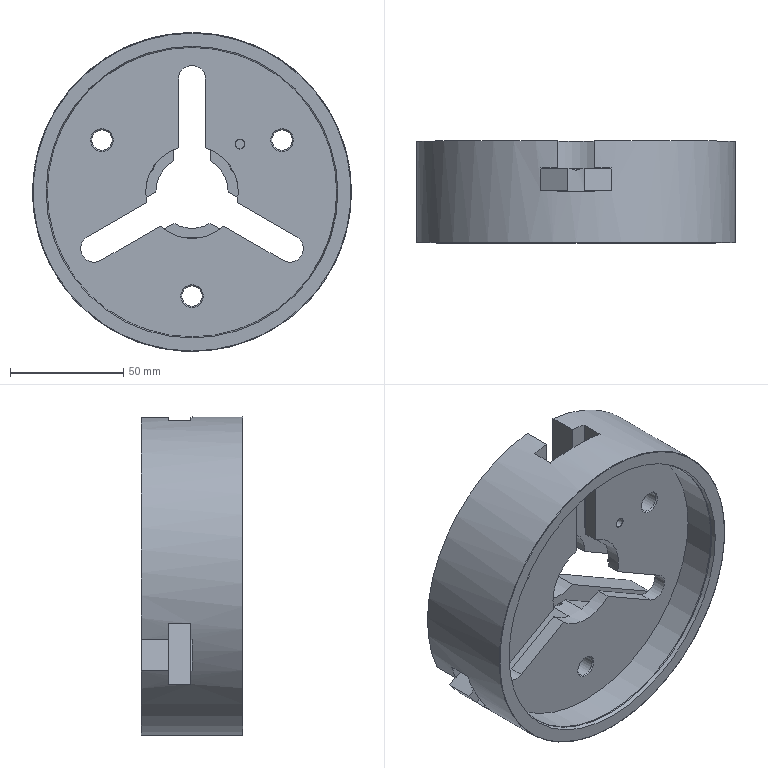NC program | NX | posted with a generic post | part box 141 x 45 x 141 mm
Whole program:
N10 G17 G21 G94 G90
(DRILLING , TOOL : D4)
N12 T01 M6
N14 G54
N16 G17 G0 G90 X0. Y-22. S3000 M3
N18 G43 Z100. H1
N20 G94 G81 G98 Z-2. F500. R3.
N22 X-19.053 Y11.
N24 X19.053
N26 X39.837 Y23.
N28 X0. Y-46.
N30 X-39.837 Y23.
N32 G80
N34 G0 X-39.837 Y23. Z100.
N36 M5
(PECK_DRILLING , TOOL : D4.2)
N38 T02 M6
N40 G54
N42 G17 G0 G90 X0. Y-22. S1600 M3
N44 G43 Z100. H2
N46 G95 G83 G98 Z-12.5 F200. Q2. R3.
N48 X19.053 Y11.
N50 X-19.053
N52 G80
N54 G0 X-19.053 Y11. Z100.
N56 M5
(PECK_DRILLING_1 , TOOL : D9)
N58 T03 M6
N60 G54
N62 G17 G0 G90 X0. Y-46. S1200 M3
N64 G43 Z100. H3
N66 G95 G83 G98 Z-32. F160. Q2. R3.
N68 X39.837 Y23.
N70 X-39.837
N72 G80
N74 G0 X-39.837 Y23. Z100.
N76 M5
(PECK_DRILLING_1_COPY , TOOL : D14)
N78 T04 M6
N80 G54
N82 G17 G0 G90 X0. Y-46. S1200 M3
N84 G43 Z100. H4
N86 G95 G83 G98 Z-8.5 F100. Q2. R3.
N88 X39.837 Y23.
N90 X-39.837
N92 G80
N94 G0 X-39.837 Y23. Z100.
N96 M5
N98 M2